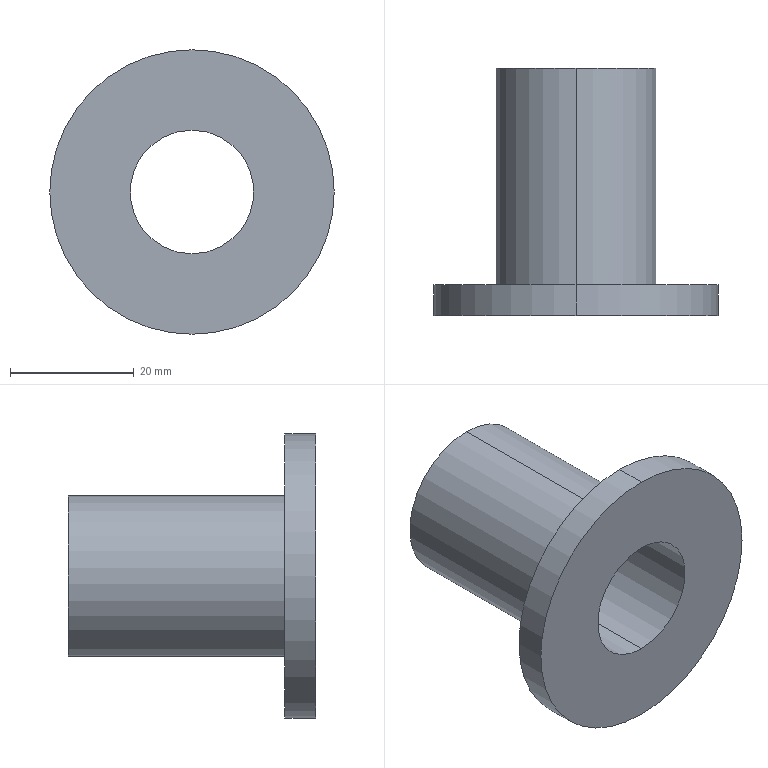Part | SolidWorks | features Revolution 1 | 1 solid | 9 faces | box 46 x 40 x 46 mm | volume 14326 mm3 | cylinder 6 | plane 3 | commonest cylinder face diameters 20 x2 26 x2 46 x2
STEP:
#1=CARTESIAN_POINT('',(0.,40.,-13.));
#2=VERTEX_POINT('',#1);
#3=CARTESIAN_POINT('',(0.,40.,13.));
#4=VERTEX_POINT('',#3);
#5=CARTESIAN_POINT('',(0.,40.,0.));
#6=DIRECTION('',(0.,-1.,0.));
#7=DIRECTION('',(0.,0.,-1.));
#8=AXIS2_PLACEMENT_3D('',#5,#6,#7);
#9=CIRCLE('',#8,13.);
#10=EDGE_CURVE('',#2,#4,#9,.T.);
#11=ORIENTED_EDGE('',*,*,#10,.T.);
#12=CARTESIAN_POINT('',(0.,5.,13.));
#13=VERTEX_POINT('',#12);
#14=CARTESIAN_POINT('',(0.,0.,13.));
#15=DIRECTION('',(0.,-1.,0.));
#16=VECTOR('',#15,1000.);
#17=LINE('',#14,#16);
#18=EDGE_CURVE('',#4,#13,#17,.T.);
#19=ORIENTED_EDGE('',*,*,#18,.T.);
#20=CARTESIAN_POINT('',(0.,5.,-13.));
#21=VERTEX_POINT('',#20);
#22=CARTESIAN_POINT('',(0.,5.,0.));
#23=DIRECTION('',(0.,-1.,0.));
#24=DIRECTION('',(0.,0.,-1.));
#25=AXIS2_PLACEMENT_3D('',#22,#23,#24);
#26=CIRCLE('',#25,13.);
#27=EDGE_CURVE('',#21,#13,#26,.T.);
#28=ORIENTED_EDGE('',*,*,#27,.F.);
#29=CARTESIAN_POINT('',(0.,0.,-13.));
#30=DIRECTION('',(0.,-1.,0.));
#31=VECTOR('',#30,1000.);
#32=LINE('',#29,#31);
#33=EDGE_CURVE('',#2,#21,#32,.T.);
#34=ORIENTED_EDGE('',*,*,#33,.F.);
#35=EDGE_LOOP('',(#11,#19,#28,#34));
#36=FACE_OUTER_BOUND('',#35,.T.);
#37=CARTESIAN_POINT('',(0.,0.,0.));
#38=DIRECTION('',(0.,-1.,0.));
#39=DIRECTION('',(0.,0.,-1.));
#40=AXIS2_PLACEMENT_3D('',#37,#38,#39);
#41=CYLINDRICAL_SURFACE('',#40,13.);
#42=ADVANCED_FACE('',(#36),#41,.T.);
#43=CARTESIAN_POINT('',(0.,5.,-23.));
#44=VERTEX_POINT('',#43);
#45=CARTESIAN_POINT('',(0.,5.,23.));
#46=VERTEX_POINT('',#45);
#47=CARTESIAN_POINT('',(0.,5.,0.));
#48=DIRECTION('',(0.,-1.,0.));
#49=DIRECTION('',(0.,0.,-1.));
#50=AXIS2_PLACEMENT_3D('',#47,#48,#49);
#51=CIRCLE('',#50,23.);
#52=EDGE_CURVE('',#44,#46,#51,.T.);
#53=ORIENTED_EDGE('',*,*,#52,.T.);
#54=CARTESIAN_POINT('',(0.,0.,23.));
#55=VERTEX_POINT('',#54);
#56=CARTESIAN_POINT('',(0.,0.,23.));
#57=DIRECTION('',(0.,-1.,0.));
#58=VECTOR('',#57,1000.);
#59=LINE('',#56,#58);
#60=EDGE_CURVE('',#46,#55,#59,.T.);
#61=ORIENTED_EDGE('',*,*,#60,.T.);
#62=CARTESIAN_POINT('',(0.,0.,-23.));
#63=VERTEX_POINT('',#62);
#64=CARTESIAN_POINT('',(0.,0.,0.));
#65=DIRECTION('',(0.,-1.,0.));
#66=DIRECTION('',(0.,0.,-1.));
#67=AXIS2_PLACEMENT_3D('',#64,#65,#66);
#68=CIRCLE('',#67,23.);
#69=EDGE_CURVE('',#63,#55,#68,.T.);
#70=ORIENTED_EDGE('',*,*,#69,.F.);
#71=CARTESIAN_POINT('',(0.,0.,-23.));
#72=DIRECTION('',(0.,-1.,0.));
#73=VECTOR('',#72,1000.);
#74=LINE('',#71,#73);
#75=EDGE_CURVE('',#44,#63,#74,.T.);
#76=ORIENTED_EDGE('',*,*,#75,.F.);
#77=EDGE_LOOP('',(#53,#61,#70,#76));
#78=FACE_OUTER_BOUND('',#77,.T.);
#79=CARTESIAN_POINT('',(0.,0.,0.));
#80=DIRECTION('',(0.,-1.,0.));
#81=DIRECTION('',(0.,0.,-1.));
#82=AXIS2_PLACEMENT_3D('',#79,#80,#81);
#83=CYLINDRICAL_SURFACE('',#82,23.);
#84=ADVANCED_FACE('',(#78),#83,.T.);
#85=CARTESIAN_POINT('',(0.,40.,10.));
#86=VERTEX_POINT('',#85);
#87=CARTESIAN_POINT('',(0.,40.,-10.));
#88=VERTEX_POINT('',#87);
#89=CARTESIAN_POINT('',(0.,40.,0.));
#90=DIRECTION('',(0.,-1.,0.));
#91=DIRECTION('',(0.,0.,-1.));
#92=AXIS2_PLACEMENT_3D('',#89,#90,#91);
#93=CIRCLE('',#92,10.);
#94=EDGE_CURVE('',#86,#88,#93,.T.);
#95=ORIENTED_EDGE('',*,*,#94,.F.);
#96=CARTESIAN_POINT('',(0.,0.,10.));
#97=VERTEX_POINT('',#96);
#98=CARTESIAN_POINT('',(0.,0.,10.));
#99=DIRECTION('',(0.,-1.,0.));
#100=VECTOR('',#99,1000.);
#101=LINE('',#98,#100);
#102=EDGE_CURVE('',#86,#97,#101,.T.);
#103=ORIENTED_EDGE('',*,*,#102,.T.);
#104=CARTESIAN_POINT('',(0.,0.,-10.));
#105=VERTEX_POINT('',#104);
#106=CARTESIAN_POINT('',(0.,0.,0.));
#107=DIRECTION('',(0.,-1.,0.));
#108=DIRECTION('',(0.,0.,-1.));
#109=AXIS2_PLACEMENT_3D('',#106,#107,#108);
#110=CIRCLE('',#109,10.);
#111=EDGE_CURVE('',#97,#105,#110,.T.);
#112=ORIENTED_EDGE('',*,*,#111,.T.);
#113=CARTESIAN_POINT('',(0.,0.,-10.));
#114=DIRECTION('',(0.,-1.,0.));
#115=VECTOR('',#114,1000.);
#116=LINE('',#113,#115);
#117=EDGE_CURVE('',#88,#105,#116,.T.);
#118=ORIENTED_EDGE('',*,*,#117,.F.);
#119=EDGE_LOOP('',(#95,#103,#112,#118));
#120=FACE_OUTER_BOUND('',#119,.T.);
#121=CARTESIAN_POINT('',(0.,0.,0.));
#122=DIRECTION('',(0.,-1.,0.));
#123=DIRECTION('',(0.,0.,-1.));
#124=AXIS2_PLACEMENT_3D('',#121,#122,#123);
#125=CYLINDRICAL_SURFACE('',#124,10.);
#126=ADVANCED_FACE('',(#120),#125,.F.);
#127=ORIENTED_EDGE('',*,*,#102,.F.);
#128=CARTESIAN_POINT('',(0.,40.,0.));
#129=DIRECTION('',(0.,-1.,0.));
#130=DIRECTION('',(0.,0.,-1.));
#131=AXIS2_PLACEMENT_3D('',#128,#129,#130);
#132=CIRCLE('',#131,10.);
#133=EDGE_CURVE('',#88,#86,#132,.T.);
#134=ORIENTED_EDGE('',*,*,#133,.F.);
#135=ORIENTED_EDGE('',*,*,#117,.T.);
#136=CARTESIAN_POINT('',(0.,0.,0.));
#137=DIRECTION('',(0.,-1.,0.));
#138=DIRECTION('',(0.,0.,-1.));
#139=AXIS2_PLACEMENT_3D('',#136,#137,#138);
#140=CIRCLE('',#139,10.);
#141=EDGE_CURVE('',#105,#97,#140,.T.);
#142=ORIENTED_EDGE('',*,*,#141,.T.);
#143=EDGE_LOOP('',(#127,#134,#135,#142));
#144=FACE_OUTER_BOUND('',#143,.T.);
#145=CARTESIAN_POINT('',(0.,0.,0.));
#146=DIRECTION('',(0.,-1.,0.));
#147=DIRECTION('',(0.,0.,-1.));
#148=AXIS2_PLACEMENT_3D('',#145,#146,#147);
#149=CYLINDRICAL_SURFACE('',#148,10.);
#150=ADVANCED_FACE('',(#144),#149,.F.);
#151=ORIENTED_EDGE('',*,*,#141,.F.);
#152=ORIENTED_EDGE('',*,*,#111,.F.);
#153=EDGE_LOOP('',(#151,#152));
#154=FACE_BOUND('',#153,.T.);
#155=ORIENTED_EDGE('',*,*,#69,.T.);
#156=CARTESIAN_POINT('',(0.,0.,0.));
#157=DIRECTION('',(0.,-1.,0.));
#158=DIRECTION('',(0.,0.,-1.));
#159=AXIS2_PLACEMENT_3D('',#156,#157,#158);
#160=CIRCLE('',#159,23.);
#161=EDGE_CURVE('',#55,#63,#160,.T.);
#162=ORIENTED_EDGE('',*,*,#161,.T.);
#163=EDGE_LOOP('',(#155,#162));
#164=FACE_OUTER_BOUND('',#163,.T.);
#165=CARTESIAN_POINT('',(-10.,0.,0.));
#166=DIRECTION('',(0.,1.,0.));
#167=DIRECTION('',(0.,0.,1.));
#168=AXIS2_PLACEMENT_3D('',#165,#166,#167);
#169=PLANE('',#168);
#170=ADVANCED_FACE('',(#154,#164),#169,.F.);
#171=ORIENTED_EDGE('',*,*,#60,.F.);
#172=CARTESIAN_POINT('',(0.,5.,0.));
#173=DIRECTION('',(0.,-1.,0.));
#174=DIRECTION('',(0.,0.,-1.));
#175=AXIS2_PLACEMENT_3D('',#172,#173,#174);
#176=CIRCLE('',#175,23.);
#177=EDGE_CURVE('',#46,#44,#176,.T.);
#178=ORIENTED_EDGE('',*,*,#177,.T.);
#179=ORIENTED_EDGE('',*,*,#75,.T.);
#180=ORIENTED_EDGE('',*,*,#161,.F.);
#181=EDGE_LOOP('',(#171,#178,#179,#180));
#182=FACE_OUTER_BOUND('',#181,.T.);
#183=CARTESIAN_POINT('',(0.,0.,0.));
#184=DIRECTION('',(0.,-1.,0.));
#185=DIRECTION('',(0.,0.,-1.));
#186=AXIS2_PLACEMENT_3D('',#183,#184,#185);
#187=CYLINDRICAL_SURFACE('',#186,23.);
#188=ADVANCED_FACE('',(#182),#187,.T.);
#189=ORIENTED_EDGE('',*,*,#52,.F.);
#190=ORIENTED_EDGE('',*,*,#177,.F.);
#191=EDGE_LOOP('',(#189,#190));
#192=FACE_OUTER_BOUND('',#191,.T.);
#193=ORIENTED_EDGE('',*,*,#27,.T.);
#194=CARTESIAN_POINT('',(0.,5.,0.));
#195=DIRECTION('',(0.,-1.,0.));
#196=DIRECTION('',(0.,0.,-1.));
#197=AXIS2_PLACEMENT_3D('',#194,#195,#196);
#198=CIRCLE('',#197,13.);
#199=EDGE_CURVE('',#13,#21,#198,.T.);
#200=ORIENTED_EDGE('',*,*,#199,.T.);
#201=EDGE_LOOP('',(#193,#200));
#202=FACE_BOUND('',#201,.T.);
#203=CARTESIAN_POINT('',(-23.,5.,0.));
#204=DIRECTION('',(0.,-1.,0.));
#205=DIRECTION('',(0.,0.,-1.));
#206=AXIS2_PLACEMENT_3D('',#203,#204,#205);
#207=PLANE('',#206);
#208=ADVANCED_FACE('',(#192,#202),#207,.F.);
#209=ORIENTED_EDGE('',*,*,#18,.F.);
#210=CARTESIAN_POINT('',(0.,40.,0.));
#211=DIRECTION('',(0.,-1.,0.));
#212=DIRECTION('',(0.,0.,-1.));
#213=AXIS2_PLACEMENT_3D('',#210,#211,#212);
#214=CIRCLE('',#213,13.);
#215=EDGE_CURVE('',#4,#2,#214,.T.);
#216=ORIENTED_EDGE('',*,*,#215,.T.);
#217=ORIENTED_EDGE('',*,*,#33,.T.);
#218=ORIENTED_EDGE('',*,*,#199,.F.);
#219=EDGE_LOOP('',(#209,#216,#217,#218));
#220=FACE_OUTER_BOUND('',#219,.T.);
#221=CARTESIAN_POINT('',(0.,0.,0.));
#222=DIRECTION('',(0.,-1.,0.));
#223=DIRECTION('',(0.,0.,-1.));
#224=AXIS2_PLACEMENT_3D('',#221,#222,#223);
#225=CYLINDRICAL_SURFACE('',#224,13.);
#226=ADVANCED_FACE('',(#220),#225,.T.);
#227=ORIENTED_EDGE('',*,*,#10,.F.);
#228=ORIENTED_EDGE('',*,*,#215,.F.);
#229=EDGE_LOOP('',(#227,#228));
#230=FACE_OUTER_BOUND('',#229,.T.);
#231=ORIENTED_EDGE('',*,*,#133,.T.);
#232=ORIENTED_EDGE('',*,*,#94,.T.);
#233=EDGE_LOOP('',(#231,#232));
#234=FACE_BOUND('',#233,.T.);
#235=CARTESIAN_POINT('',(-13.,40.,0.));
#236=DIRECTION('',(0.,-1.,0.));
#237=DIRECTION('',(0.,0.,-1.));
#238=AXIS2_PLACEMENT_3D('',#235,#236,#237);
#239=PLANE('',#238);
#240=ADVANCED_FACE('',(#230,#234),#239,.F.);
#241=CLOSED_SHELL('',(#42,#84,#126,#150,#170,#188,#208,#226,#240));
#242=MANIFOLD_SOLID_BREP('',#241);
#243=CARTESIAN_POINT('',(0.,0.,0.));
#244=DIRECTION('',(0.,0.,1.));
#245=DIRECTION('',(1.,0.,0.));
#246=AXIS2_PLACEMENT_3D('',#243,#244,#245);
#247=(LENGTH_UNIT()NAMED_UNIT(*)SI_UNIT(.MILLI.,.METRE.));
#248=UNCERTAINTY_MEASURE_WITH_UNIT(LENGTH_MEASURE(0.00001),#247,'','');
#249=(NAMED_UNIT(*)PLANE_ANGLE_UNIT()SI_UNIT($,.RADIAN.));
#250=(NAMED_UNIT(*)SI_UNIT($,.STERADIAN.)SOLID_ANGLE_UNIT());
#251=(GEOMETRIC_REPRESENTATION_CONTEXT(3)GLOBAL_UNCERTAINTY_ASSIGNED_CONTEXT((#248))GLOBAL_UNIT_ASSIGNED_CONTEXT((#247,#249,#250))REPRESENTATION_CONTEXT('',''));
#252=ADVANCED_BREP_SHAPE_REPRESENTATION('',(#242,#246),#251);